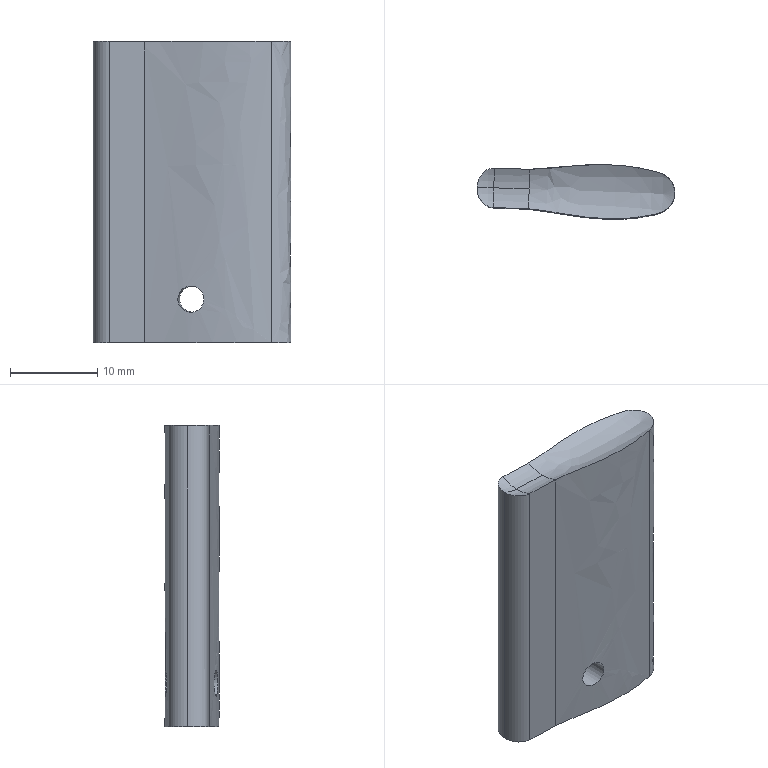Part | NX | features DIE-10 2 | 1 solid | 13 faces | volume 3861 mm3 | spline 9 | plane 3 | cylinder 1 | commonest cylinder face diameters 3 x1
STEP:
#1=CARTESIAN_POINT('',(2369.211,-905.218,828.769));
#2=VERTEX_POINT('',#1);
#3=CARTESIAN_POINT('',(2368.841,-905.228,829.937));
#4=CARTESIAN_POINT('',(2369.375,-905.214,828.774));
#5=CARTESIAN_POINT('',(2368.924,-905.225,827.579));
#6=CARTESIAN_POINT('',(2367.764,-905.286,827.056));
#7=CARTESIAN_POINT('',(2366.574,-905.393,827.498));
#8=CARTESIAN_POINT('',(2366.039,-905.455,828.658));
#9=CARTESIAN_POINT('',(2366.49,-905.402,829.851));
#10=CARTESIAN_POINT('',(2367.646,-905.295,830.376));
#11=CARTESIAN_POINT('',(2368.841,-905.228,829.937));
#12=CARTESIAN_POINT('',(2369.375,-905.214,828.774));
#13=CARTESIAN_POINT('',(2368.924,-905.225,827.579));
#14=B_SPLINE_CURVE_WITH_KNOTS('',3,(#3,#4,#5,#6,#7,#8,#9,#10,#11,#12,#13),.UNSPECIFIED.,.T.,.F.,(1,1,1,1,1,1,1,1,1,1,1,1,1,1,1),(-0.003528,-0.002352,-0.001176,0.,0.001176,0.002352,0.003528,0.004703,0.005879,0.007055,0.008231,0.009407,0.01058,0.01176,0.01293),.UNSPECIFIED.);
#15=EDGE_CURVE('',#2,#2,#14,.F.);
#16=ORIENTED_EDGE('',*,*,#15,.T.);
#17=EDGE_LOOP('',(#16));
#18=FACE_BOUND('',#17,.T.);
#19=CARTESIAN_POINT('',(2362.336,-905.735,858.258));
#20=VERTEX_POINT('',#19);
#21=CARTESIAN_POINT('',(2362.326,-905.735,823.716));
#22=VERTEX_POINT('',#21);
#23=CARTESIAN_POINT('',(2362.326,-905.735,823.716));
#24=CARTESIAN_POINT('',(2362.326,-905.735,835.23));
#25=CARTESIAN_POINT('',(2362.326,-905.735,846.744));
#26=CARTESIAN_POINT('',(2362.326,-905.735,858.258));
#27=B_SPLINE_CURVE_WITH_KNOTS('',3,(#23,#24,#25,#26),.UNSPECIFIED.,.F.,.F.,(4,4),(0.5008,0.5009),.UNSPECIFIED.);
#28=EDGE_CURVE('',#20,#22,#27,.F.);
#29=ORIENTED_EDGE('',*,*,#28,.F.);
#30=CARTESIAN_POINT('',(2376.717,-910.889,858.242));
#31=VERTEX_POINT('',#30);
#32=CARTESIAN_POINT('',(2362.326,-905.733,858.259));
#33=CARTESIAN_POINT('',(2364.117,-905.753,858.273));
#34=CARTESIAN_POINT('',(2366.78,-905.29,858.242));
#35=CARTESIAN_POINT('',(2370.346,-905.165,858.25));
#36=CARTESIAN_POINT('',(2372.574,-905.26,858.245));
#37=CARTESIAN_POINT('',(2374.365,-905.458,858.245));
#38=CARTESIAN_POINT('',(2375.69,-905.739,858.242));
#39=CARTESIAN_POINT('',(2377.015,-906.006,858.242));
#40=CARTESIAN_POINT('',(2378.275,-906.597,858.245));
#41=CARTESIAN_POINT('',(2379.025,-907.857,858.249));
#42=CARTESIAN_POINT('',(2378.948,-909.291,858.252));
#43=CARTESIAN_POINT('',(2378.038,-910.428,858.242));
#44=CARTESIAN_POINT('',(2377.168,-910.778,858.243));
#45=CARTESIAN_POINT('',(2376.717,-910.889,858.242));
#46=B_SPLINE_CURVE_WITH_KNOTS('',3,(#32,#33,#34,#35,#36,#37,#38,#39,#40,#41,#42,#43,#44,#45),.UNSPECIFIED.,.F.,.F.,(4,1,1,1,1,1,1,1,1,1,1,4),(0.,0.005363,0.008044,0.01073,0.01207,0.01341,0.01475,0.01609,0.01743,0.01877,0.02011,0.02145),.UNSPECIFIED.);
#47=EDGE_CURVE('',#20,#31,#46,.T.);
#48=ORIENTED_EDGE('',*,*,#47,.T.);
#49=CARTESIAN_POINT('',(2376.717,-910.889,823.716));
#50=VERTEX_POINT('',#49);
#51=CARTESIAN_POINT('',(2376.717,-910.889,841.133));
#52=DIRECTION('',(0.,0.,-1.));
#53=VECTOR('',#52,1000.);
#54=LINE('',#51,#53);
#55=EDGE_CURVE('',#31,#50,#54,.T.);
#56=ORIENTED_EDGE('',*,*,#55,.T.);
#57=CARTESIAN_POINT('',(2376.717,-910.889,823.716));
#58=CARTESIAN_POINT('',(2377.157,-910.781,823.716));
#59=CARTESIAN_POINT('',(2378.004,-910.446,823.716));
#60=CARTESIAN_POINT('',(2378.916,-909.351,823.716));
#61=CARTESIAN_POINT('',(2379.041,-907.939,823.716));
#62=CARTESIAN_POINT('',(2378.354,-906.687,823.716));
#63=CARTESIAN_POINT('',(2377.143,-906.031,823.716));
#64=CARTESIAN_POINT('',(2375.357,-905.671,823.716));
#65=CARTESIAN_POINT('',(2373.14,-905.263,823.716));
#66=CARTESIAN_POINT('',(2370.412,-905.171,823.716));
#67=CARTESIAN_POINT('',(2366.815,-905.282,823.716));
#68=CARTESIAN_POINT('',(2364.119,-905.753,823.716));
#69=CARTESIAN_POINT('',(2362.326,-905.733,823.716));
#70=B_SPLINE_CURVE_WITH_KNOTS('',3,(#57,#58,#59,#60,#61,#62,#63,#64,#65,#66,#67,#68,#69),.UNSPECIFIED.,.F.,.F.,(4,1,1,1,1,1,1,1,1,1,4),(0.02457,0.02592,0.02728,0.02864,0.03,0.03136,0.03272,0.03544,0.03816,0.04087,0.04631),.UNSPECIFIED.);
#71=EDGE_CURVE('',#50,#22,#70,.T.);
#72=ORIENTED_EDGE('',*,*,#71,.T.);
#73=EDGE_LOOP('',(#29,#48,#56,#72));
#74=FACE_BOUND('',#73,.T.);
#75=CARTESIAN_POINT('',(2362.17,-905.731,858.466));
#76=CARTESIAN_POINT('',(2362.17,-905.731,823.505));
#77=CARTESIAN_POINT('',(2363.26,-905.749,858.475));
#78=CARTESIAN_POINT('',(2363.26,-905.749,823.513));
#79=CARTESIAN_POINT('',(2365.476,-905.528,858.464));
#80=CARTESIAN_POINT('',(2365.476,-905.528,823.503));
#81=CARTESIAN_POINT('',(2368.424,-905.2,858.469));
#82=CARTESIAN_POINT('',(2368.424,-905.2,823.508));
#83=CARTESIAN_POINT('',(2371.439,-905.18,858.468));
#84=CARTESIAN_POINT('',(2371.439,-905.18,823.507));
#85=CARTESIAN_POINT('',(2373.938,-905.364,858.469));
#86=CARTESIAN_POINT('',(2373.938,-905.364,823.508));
#87=CARTESIAN_POINT('',(2375.811,-905.764,858.467));
#88=CARTESIAN_POINT('',(2375.811,-905.764,823.505));
#89=CARTESIAN_POINT('',(2377.335,-906.1,858.467));
#90=CARTESIAN_POINT('',(2377.335,-906.1,823.506));
#91=CARTESIAN_POINT('',(2378.205,-906.616,858.465));
#92=CARTESIAN_POINT('',(2378.205,-906.616,823.504));
#93=CARTESIAN_POINT('',(2378.888,-907.59,858.467));
#94=CARTESIAN_POINT('',(2378.888,-907.59,823.506));
#95=CARTESIAN_POINT('',(2379.023,-908.675,858.467));
#96=CARTESIAN_POINT('',(2379.023,-908.675,823.505));
#97=CARTESIAN_POINT('',(2378.683,-909.662,858.466));
#98=CARTESIAN_POINT('',(2378.683,-909.662,823.504));
#99=CARTESIAN_POINT('',(2377.849,-910.512,858.465));
#100=CARTESIAN_POINT('',(2377.849,-910.512,823.504));
#101=CARTESIAN_POINT('',(2377.168,-910.778,858.467));
#102=CARTESIAN_POINT('',(2377.168,-910.778,823.505));
#103=CARTESIAN_POINT('',(2376.717,-910.889,858.467));
#104=CARTESIAN_POINT('',(2376.717,-910.889,823.506));
#105=B_SPLINE_SURFACE_WITH_KNOTS('',3,1,((#75,#76),(#77,#78),(#79,#80),(#81,#82),(#83,#84),(#85,#86),(#87,#88),(#89,#90),(#91,#92),(#93,#94),(#95,#96),(#97,#98),(#99,#100),(#101,#102),(#103,#104)),.SURF_OF_LINEAR_EXTRUSION.,.F.,.F.,.F.,(4,1,1,1,1,1,1,1,1,1,1,1,4),(2,2),(-0.00628,0.1193,0.2448,0.3704,0.4959,0.5587,0.6215,0.6843,0.747,0.8098,0.8726,0.9354,0.9981),(0.,1.),.UNSPECIFIED.);
#106=ADVANCED_FACE('',(#18,#74),#105,.T.);
#107=CARTESIAN_POINT('',(2369.,-911.248,828.769));
#108=VERTEX_POINT('',#107);
#109=CARTESIAN_POINT('',(2368.714,-911.221,827.578));
#110=CARTESIAN_POINT('',(2369.164,-911.264,828.775));
#111=CARTESIAN_POINT('',(2368.633,-911.213,829.935));
#112=CARTESIAN_POINT('',(2367.447,-911.063,830.376));
#113=CARTESIAN_POINT('',(2366.3,-910.873,829.853));
#114=CARTESIAN_POINT('',(2365.853,-910.788,828.658));
#115=CARTESIAN_POINT('',(2366.38,-910.888,827.5));
#116=CARTESIAN_POINT('',(2367.559,-911.079,827.056));
#117=CARTESIAN_POINT('',(2368.714,-911.221,827.578));
#118=CARTESIAN_POINT('',(2369.164,-911.264,828.775));
#119=CARTESIAN_POINT('',(2368.633,-911.213,829.935));
#120=B_SPLINE_CURVE_WITH_KNOTS('',3,(#109,#110,#111,#112,#113,#114,#115,#116,#117,#118,#119),.UNSPECIFIED.,.T.,.F.,(1,1,1,1,1,1,1,1,1,1,1,1,1,1,1),(-0.003528,-0.002352,-0.001176,0.,0.001176,0.002352,0.003528,0.004704,0.005879,0.007055,0.008231,0.009407,0.01058,0.01176,0.01293),.UNSPECIFIED.);
#121=EDGE_CURVE('',#108,#108,#120,.F.);
#122=ORIENTED_EDGE('',*,*,#121,.T.);
#123=EDGE_LOOP('',(#122));
#124=FACE_BOUND('',#123,.T.);
#125=ORIENTED_EDGE('',*,*,#55,.F.);
#126=CARTESIAN_POINT('',(2362.184,-910.261,858.258));
#127=VERTEX_POINT('',#126);
#128=CARTESIAN_POINT('',(2376.717,-910.889,858.242));
#129=CARTESIAN_POINT('',(2375.519,-911.158,858.226));
#130=CARTESIAN_POINT('',(2373.113,-911.498,858.253));
#131=CARTESIAN_POINT('',(2369.446,-911.36,858.244));
#132=CARTESIAN_POINT('',(2365.815,-910.809,858.245));
#133=CARTESIAN_POINT('',(2363.413,-910.336,858.267));
#134=CARTESIAN_POINT('',(2362.189,-910.262,858.258));
#135=B_SPLINE_CURVE_WITH_KNOTS('',3,(#128,#129,#130,#131,#132,#133,#134),.UNSPECIFIED.,.F.,.F.,(4,1,1,1,4),(0.,0.003638,0.007277,0.01092,0.01455),.UNSPECIFIED.);
#136=EDGE_CURVE('',#31,#127,#135,.T.);
#137=ORIENTED_EDGE('',*,*,#136,.T.);
#138=CARTESIAN_POINT('',(2362.185,-910.261,857.716));
#139=VERTEX_POINT('',#138);
#140=CARTESIAN_POINT('',(2362.179,-910.261,857.716));
#141=CARTESIAN_POINT('',(2362.179,-910.261,857.897));
#142=CARTESIAN_POINT('',(2362.179,-910.261,858.078));
#143=CARTESIAN_POINT('',(2362.179,-910.261,858.258));
#144=B_SPLINE_CURVE_WITH_KNOTS('',3,(#140,#141,#142,#143),.UNSPECIFIED.,.F.,.F.,(4,4),(0.,0.3599),.UNSPECIFIED.);
#145=EDGE_CURVE('',#127,#139,#144,.F.);
#146=ORIENTED_EDGE('',*,*,#145,.T.);
#147=CARTESIAN_POINT('',(2362.196,-910.262,823.716));
#148=VERTEX_POINT('',#147);
#149=CARTESIAN_POINT('',(2362.202,-910.262,823.716));
#150=CARTESIAN_POINT('',(2362.199,-910.261,835.05));
#151=CARTESIAN_POINT('',(2362.195,-910.261,846.383));
#152=CARTESIAN_POINT('',(2362.192,-910.261,857.716));
#153=B_SPLINE_CURVE_WITH_KNOTS('',3,(#149,#150,#151,#152),.UNSPECIFIED.,.F.,.F.,(4,4),(0.,1.),.UNSPECIFIED.);
#154=EDGE_CURVE('',#139,#148,#153,.F.);
#155=ORIENTED_EDGE('',*,*,#154,.T.);
#156=CARTESIAN_POINT('',(2362.196,-910.262,823.716));
#157=CARTESIAN_POINT('',(2363.419,-910.337,823.716));
#158=CARTESIAN_POINT('',(2365.818,-910.807,823.716));
#159=CARTESIAN_POINT('',(2370.65,-911.555,823.716));
#160=CARTESIAN_POINT('',(2374.335,-911.423,823.716));
#161=CARTESIAN_POINT('',(2376.717,-910.889,823.716));
#162=B_SPLINE_CURVE_WITH_KNOTS('',3,(#156,#157,#158,#159,#160,#161),.UNSPECIFIED.,.F.,.F.,(4,1,1,4),(0.02991,0.03359,0.03727,0.04462),.UNSPECIFIED.);
#163=EDGE_CURVE('',#148,#50,#162,.T.);
#164=ORIENTED_EDGE('',*,*,#163,.T.);
#165=EDGE_LOOP('',(#125,#137,#146,#155,#164));
#166=FACE_BOUND('',#165,.T.);
#167=CARTESIAN_POINT('',(2376.717,-910.889,858.483));
#168=CARTESIAN_POINT('',(2376.717,-910.889,823.509));
#169=CARTESIAN_POINT('',(2376.089,-911.03,858.483));
#170=CARTESIAN_POINT('',(2376.089,-911.03,823.509));
#171=CARTESIAN_POINT('',(2374.973,-911.262,858.484));
#172=CARTESIAN_POINT('',(2374.973,-911.262,823.509));
#173=CARTESIAN_POINT('',(2372.578,-911.457,858.484));
#174=CARTESIAN_POINT('',(2372.578,-911.457,823.509));
#175=CARTESIAN_POINT('',(2369.574,-911.374,858.484));
#176=CARTESIAN_POINT('',(2369.574,-911.374,823.509));
#177=CARTESIAN_POINT('',(2365.952,-910.842,858.483));
#178=CARTESIAN_POINT('',(2365.952,-910.842,823.508));
#179=CARTESIAN_POINT('',(2363.495,-910.342,858.483));
#180=CARTESIAN_POINT('',(2363.495,-910.342,823.509));
#181=CARTESIAN_POINT('',(2362.077,-910.255,858.483));
#182=CARTESIAN_POINT('',(2362.077,-910.255,823.509));
#183=B_SPLINE_SURFACE_WITH_KNOTS('',3,1,((#167,#168),(#169,#170),(#171,#172),(#173,#174),(#175,#176),(#177,#178),(#179,#180),(#181,#182)),.SURF_OF_LINEAR_EXTRUSION.,.F.,.F.,.F.,(4,1,1,1,1,4),(2,2),(-0.002152,0.124,0.2502,0.5026,0.755,1.007),(0.,1.),.UNSPECIFIED.);
#184=ADVANCED_FACE('',(#124,#166),#183,.T.);
#185=CARTESIAN_POINT('',(2358.287,-905.594,858.258));
#186=VERTEX_POINT('',#185);
#187=CARTESIAN_POINT('',(2358.286,-905.594,823.716));
#188=VERTEX_POINT('',#187);
#189=CARTESIAN_POINT('',(2358.287,-905.594,858.258));
#190=CARTESIAN_POINT('',(2358.287,-905.594,846.744));
#191=CARTESIAN_POINT('',(2358.287,-905.594,835.23));
#192=CARTESIAN_POINT('',(2358.287,-905.594,823.716));
#193=B_SPLINE_CURVE_WITH_KNOTS('',3,(#189,#190,#191,#192),.UNSPECIFIED.,.F.,.F.,(4,4),(0.4991,0.4992),.UNSPECIFIED.);
#194=EDGE_CURVE('',#186,#188,#193,.T.);
#195=ORIENTED_EDGE('',*,*,#194,.F.);
#196=CARTESIAN_POINT('',(2358.287,-905.594,858.258));
#197=CARTESIAN_POINT('',(2359.636,-905.641,858.258));
#198=CARTESIAN_POINT('',(2360.986,-905.689,858.258));
#199=CARTESIAN_POINT('',(2362.335,-905.736,858.258));
#200=B_SPLINE_CURVE_WITH_KNOTS('',3,(#196,#197,#198,#199),.UNSPECIFIED.,.F.,.F.,(4,4),(0.,0.004051),.UNSPECIFIED.);
#201=EDGE_CURVE('',#186,#20,#200,.T.);
#202=ORIENTED_EDGE('',*,*,#201,.T.);
#203=ORIENTED_EDGE('',*,*,#28,.T.);
#204=CARTESIAN_POINT('',(2362.269,-905.733,823.716));
#205=DIRECTION('',(-0.9994,0.0349,0.));
#206=VECTOR('',#205,1000.);
#207=LINE('',#204,#206);
#208=EDGE_CURVE('',#22,#188,#207,.T.);
#209=ORIENTED_EDGE('',*,*,#208,.T.);
#210=EDGE_LOOP('',(#195,#202,#203,#209));
#211=FACE_BOUND('',#210,.T.);
#212=CARTESIAN_POINT('',(2362.269,-905.733,858.55));
#213=DIRECTION('',(0.0349,0.9994,0.));
#214=DIRECTION('',(-0.9994,0.0349,0.));
#215=AXIS2_PLACEMENT_3D('',#212,#213,#214);
#216=PLANE('',#215);
#217=ADVANCED_FACE('',(#211),#216,.T.);
#218=CARTESIAN_POINT('',(2356.311,-907.791,858.196));
#219=VERTEX_POINT('',#218);
#220=CARTESIAN_POINT('',(2358.286,-905.594,858.258));
#221=CARTESIAN_POINT('',(2357.734,-905.574,858.259));
#222=CARTESIAN_POINT('',(2356.678,-906.139,858.228));
#223=CARTESIAN_POINT('',(2356.332,-907.24,858.195));
#224=CARTESIAN_POINT('',(2356.311,-907.79,858.196));
#225=B_SPLINE_CURVE_WITH_KNOTS('',3,(#220,#221,#222,#223,#224),.UNSPECIFIED.,.F.,.F.,(4,1,4),(0.,0.001633,0.003266),.UNSPECIFIED.);
#226=EDGE_CURVE('',#186,#219,#225,.T.);
#227=ORIENTED_EDGE('',*,*,#226,.F.);
#228=ORIENTED_EDGE('',*,*,#194,.T.);
#229=CARTESIAN_POINT('',(2356.311,-907.79,823.716));
#230=VERTEX_POINT('',#229);
#231=CARTESIAN_POINT('',(2358.286,-905.594,823.716));
#232=CARTESIAN_POINT('',(2357.734,-905.574,823.716));
#233=CARTESIAN_POINT('',(2356.678,-906.138,823.716));
#234=CARTESIAN_POINT('',(2356.332,-907.241,823.716));
#235=CARTESIAN_POINT('',(2356.311,-907.79,823.716));
#236=B_SPLINE_CURVE_WITH_KNOTS('',3,(#231,#232,#233,#234,#235),.UNSPECIFIED.,.F.,.F.,(4,1,4),(0.03107,0.03273,0.03439),.UNSPECIFIED.);
#237=EDGE_CURVE('',#188,#230,#236,.T.);
#238=ORIENTED_EDGE('',*,*,#237,.T.);
#239=CARTESIAN_POINT('',(2356.311,-907.793,858.196));
#240=CARTESIAN_POINT('',(2356.311,-907.793,846.703));
#241=CARTESIAN_POINT('',(2356.311,-907.793,835.21));
#242=CARTESIAN_POINT('',(2356.311,-907.793,823.716));
#243=B_SPLINE_CURVE_WITH_KNOTS('',3,(#239,#240,#241,#242),.UNSPECIFIED.,.F.,.F.,(4,4),(0.4991,0.4992),.UNSPECIFIED.);
#244=EDGE_CURVE('',#219,#230,#243,.T.);
#245=ORIENTED_EDGE('',*,*,#244,.F.);
#246=EDGE_LOOP('',(#227,#228,#238,#245));
#247=FACE_BOUND('',#246,.T.);
#248=CARTESIAN_POINT('',(2356.311,-907.793,858.432));
#249=CARTESIAN_POINT('',(2356.311,-907.793,823.476));
#250=CARTESIAN_POINT('',(2356.318,-907.615,858.432));
#251=CARTESIAN_POINT('',(2356.318,-907.615,823.476));
#252=CARTESIAN_POINT('',(2356.349,-907.359,858.433));
#253=CARTESIAN_POINT('',(2356.349,-907.359,823.477));
#254=CARTESIAN_POINT('',(2356.509,-906.778,858.439));
#255=CARTESIAN_POINT('',(2356.509,-906.778,823.482));
#256=CARTESIAN_POINT('',(2356.874,-906.172,858.451));
#257=CARTESIAN_POINT('',(2356.874,-906.172,823.494));
#258=CARTESIAN_POINT('',(2357.409,-905.766,858.46));
#259=CARTESIAN_POINT('',(2357.409,-905.766,823.504));
#260=CARTESIAN_POINT('',(2357.922,-905.61,858.465));
#261=CARTESIAN_POINT('',(2357.922,-905.61,823.508));
#262=CARTESIAN_POINT('',(2358.126,-905.588,858.466));
#263=CARTESIAN_POINT('',(2358.126,-905.588,823.509));
#264=CARTESIAN_POINT('',(2358.286,-905.594,858.465));
#265=CARTESIAN_POINT('',(2358.286,-905.594,823.509));
#266=B_SPLINE_SURFACE_WITH_KNOTS('',3,1,((#248,#249),(#250,#251),(#252,#253),(#254,#255),(#256,#257),(#258,#259),(#260,#261),(#262,#263),(#264,#265)),.SURF_OF_LINEAR_EXTRUSION.,.F.,.F.,.F.,(4,1,1,1,1,1,4),(2,2),(0.0001248,0.1252,0.2502,0.5002,0.7503,0.8753,1.),(0.,1.),.UNSPECIFIED.);
#267=ADVANCED_FACE('',(#247),#266,.T.);
#268=CARTESIAN_POINT('',(2358.132,-910.119,858.258));
#269=VERTEX_POINT('',#268);
#270=CARTESIAN_POINT('',(2358.134,-910.119,823.716));
#271=VERTEX_POINT('',#270);
#272=CARTESIAN_POINT('',(2358.134,-910.119,823.716));
#273=CARTESIAN_POINT('',(2358.134,-910.119,835.23));
#274=CARTESIAN_POINT('',(2358.134,-910.119,846.744));
#275=CARTESIAN_POINT('',(2358.134,-910.119,858.258));
#276=B_SPLINE_CURVE_WITH_KNOTS('',3,(#272,#273,#274,#275),.UNSPECIFIED.,.F.,.F.,(4,4),(0.5008,0.5009),.UNSPECIFIED.);
#277=EDGE_CURVE('',#269,#271,#276,.F.);
#278=ORIENTED_EDGE('',*,*,#277,.F.);
#279=CARTESIAN_POINT('',(2358.135,-910.119,858.258));
#280=CARTESIAN_POINT('',(2357.581,-910.099,858.258));
#281=CARTESIAN_POINT('',(2356.564,-909.466,858.228));
#282=CARTESIAN_POINT('',(2356.292,-908.341,858.196));
#283=CARTESIAN_POINT('',(2356.311,-907.79,858.196));
#284=B_SPLINE_CURVE_WITH_KNOTS('',3,(#279,#280,#281,#282,#283),.UNSPECIFIED.,.F.,.F.,(4,1,4),(0.,0.001637,0.003275),.UNSPECIFIED.);
#285=EDGE_CURVE('',#269,#219,#284,.T.);
#286=ORIENTED_EDGE('',*,*,#285,.T.);
#287=ORIENTED_EDGE('',*,*,#244,.T.);
#288=CARTESIAN_POINT('',(2358.134,-910.119,823.716));
#289=CARTESIAN_POINT('',(2357.581,-910.099,823.716));
#290=CARTESIAN_POINT('',(2356.565,-909.468,823.716));
#291=CARTESIAN_POINT('',(2356.292,-908.34,823.716));
#292=CARTESIAN_POINT('',(2356.311,-907.79,823.716));
#293=B_SPLINE_CURVE_WITH_KNOTS('',3,(#288,#289,#290,#291,#292),.UNSPECIFIED.,.F.,.F.,(4,1,4),(0.05975,0.06141,0.06307),.UNSPECIFIED.);
#294=EDGE_CURVE('',#271,#230,#293,.T.);
#295=ORIENTED_EDGE('',*,*,#294,.F.);
#296=EDGE_LOOP('',(#278,#286,#287,#295));
#297=FACE_BOUND('',#296,.T.);
#298=CARTESIAN_POINT('',(2358.135,-910.119,858.465));
#299=CARTESIAN_POINT('',(2358.135,-910.119,823.509));
#300=CARTESIAN_POINT('',(2358.035,-910.115,858.465));
#301=CARTESIAN_POINT('',(2358.035,-910.115,823.509));
#302=CARTESIAN_POINT('',(2357.955,-910.106,858.465));
#303=CARTESIAN_POINT('',(2357.955,-910.106,823.509));
#304=CARTESIAN_POINT('',(2357.678,-910.051,858.464));
#305=CARTESIAN_POINT('',(2357.678,-910.051,823.508));
#306=CARTESIAN_POINT('',(2357.279,-909.886,858.461));
#307=CARTESIAN_POINT('',(2357.279,-909.886,823.504));
#308=CARTESIAN_POINT('',(2356.755,-909.445,858.451));
#309=CARTESIAN_POINT('',(2356.755,-909.445,823.494));
#310=CARTESIAN_POINT('',(2356.375,-908.681,858.437));
#311=CARTESIAN_POINT('',(2356.375,-908.681,823.48));
#312=CARTESIAN_POINT('',(2356.3,-908.088,858.432));
#313=CARTESIAN_POINT('',(2356.3,-908.088,823.476));
#314=CARTESIAN_POINT('',(2356.311,-907.79,858.432));
#315=CARTESIAN_POINT('',(2356.311,-907.79,823.476));
#316=B_SPLINE_SURFACE_WITH_KNOTS('',3,1,((#298,#299),(#300,#301),(#302,#303),(#304,#305),(#306,#307),(#308,#309),(#310,#311),(#312,#313),(#314,#315)),.SURF_OF_LINEAR_EXTRUSION.,.F.,.F.,.F.,(4,1,1,1,1,1,4),(2,2),(0.0008005,0.06324,0.1257,0.2506,0.5003,0.7501,0.9999),(0.,1.),.UNSPECIFIED.);
#317=ADVANCED_FACE('',(#297),#316,.T.);
#318=CARTESIAN_POINT('',(2362.189,-910.261,858.258));
#319=CARTESIAN_POINT('',(2360.838,-910.214,858.258));
#320=CARTESIAN_POINT('',(2359.486,-910.167,858.258));
#321=CARTESIAN_POINT('',(2358.134,-910.119,858.258));
#322=B_SPLINE_CURVE_WITH_KNOTS('',3,(#318,#319,#320,#321),.UNSPECIFIED.,.F.,.F.,(4,4),(0.,0.004058),.UNSPECIFIED.);
#323=EDGE_CURVE('',#127,#269,#322,.T.);
#324=ORIENTED_EDGE('',*,*,#323,.F.);
#325=CARTESIAN_POINT('',(2362.273,-907.996,857.716));
#326=VERTEX_POINT('',#325);
#327=CARTESIAN_POINT('',(2362.189,-910.261,858.258));
#328=CARTESIAN_POINT('',(2362.216,-909.488,857.866));
#329=CARTESIAN_POINT('',(2362.244,-908.699,857.716));
#330=CARTESIAN_POINT('',(2362.268,-907.999,857.716));
#331=B_SPLINE_CURVE_WITH_KNOTS('',3,(#327,#328,#329,#330),.UNSPECIFIED.,.F.,.F.,(4,4),(0.1786,1.),.UNSPECIFIED.);
#332=EDGE_CURVE('',#127,#326,#331,.T.);
#333=ORIENTED_EDGE('',*,*,#332,.T.);
#334=CARTESIAN_POINT('',(2358.21,-907.856,857.716));
#335=VERTEX_POINT('',#334);
#336=CARTESIAN_POINT('',(2362.268,-907.999,857.716));
#337=CARTESIAN_POINT('',(2360.915,-907.951,857.716));
#338=CARTESIAN_POINT('',(2359.562,-907.904,857.716));
#339=CARTESIAN_POINT('',(2358.21,-907.857,857.716));
#340=B_SPLINE_CURVE_WITH_KNOTS('',3,(#336,#337,#338,#339),.UNSPECIFIED.,.F.,.F.,(4,4),(0.,0.9999),.UNSPECIFIED.);
#341=EDGE_CURVE('',#335,#326,#340,.F.);
#342=ORIENTED_EDGE('',*,*,#341,.F.);
#343=CARTESIAN_POINT('',(2358.209,-907.857,857.716));
#344=CARTESIAN_POINT('',(2358.185,-908.557,857.716));
#345=CARTESIAN_POINT('',(2358.157,-909.347,857.866));
#346=CARTESIAN_POINT('',(2358.13,-910.119,858.258));
#347=B_SPLINE_CURVE_WITH_KNOTS('',3,(#343,#344,#345,#346),.UNSPECIFIED.,.F.,.F.,(4,4),(0.,0.8214),.UNSPECIFIED.);
#348=EDGE_CURVE('',#269,#335,#347,.F.);
#349=ORIENTED_EDGE('',*,*,#348,.F.);
#350=EDGE_LOOP('',(#324,#333,#342,#349));
#351=FACE_BOUND('',#350,.T.);
#352=CARTESIAN_POINT('',(2358.209,-907.857,857.716));
#353=CARTESIAN_POINT('',(2358.185,-908.561,857.716));
#354=CARTESIAN_POINT('',(2358.157,-909.355,857.867));
#355=CARTESIAN_POINT('',(2358.13,-910.133,858.265));
#356=CARTESIAN_POINT('',(2359.562,-907.904,857.716));
#357=CARTESIAN_POINT('',(2359.538,-908.609,857.716));
#358=CARTESIAN_POINT('',(2359.51,-909.403,857.867));
#359=CARTESIAN_POINT('',(2359.483,-910.18,858.265));
#360=CARTESIAN_POINT('',(2360.915,-907.951,857.716));
#361=CARTESIAN_POINT('',(2360.891,-908.656,857.716));
#362=CARTESIAN_POINT('',(2360.863,-909.45,857.867));
#363=CARTESIAN_POINT('',(2360.836,-910.228,858.265));
#364=CARTESIAN_POINT('',(2362.268,-907.999,857.716));
#365=CARTESIAN_POINT('',(2362.244,-908.703,857.716));
#366=CARTESIAN_POINT('',(2362.216,-909.497,857.867));
#367=CARTESIAN_POINT('',(2362.189,-910.275,858.265));
#368=B_SPLINE_SURFACE_WITH_KNOTS('',3,3,((#352,#353,#354,#355),(#356,#357,#358,#359),(#360,#361,#362,#363),(#364,#365,#366,#367)),.UNSPECIFIED.,.F.,.F.,.F.,(4,4),(4,4),(0.,1.),(0.,0.8263),.UNSPECIFIED.);
#369=ADVANCED_FACE('',(#351),#368,.F.);
#370=ORIENTED_EDGE('',*,*,#47,.F.);
#371=CARTESIAN_POINT('',(2362.347,-905.736,858.258));
#372=CARTESIAN_POINT('',(2362.324,-906.365,857.939));
#373=CARTESIAN_POINT('',(2362.298,-907.139,857.717));
#374=CARTESIAN_POINT('',(2362.268,-907.995,857.716));
#375=B_SPLINE_CURVE_WITH_KNOTS('',3,(#371,#372,#373,#374),.UNSPECIFIED.,.F.,.F.,(4,4),(0.1357,1.),.UNSPECIFIED.);
#376=EDGE_CURVE('',#326,#20,#375,.F.);
#377=ORIENTED_EDGE('',*,*,#376,.F.);
#378=ORIENTED_EDGE('',*,*,#332,.F.);
#379=ORIENTED_EDGE('',*,*,#136,.F.);
#380=EDGE_LOOP('',(#370,#377,#378,#379));
#381=FACE_BOUND('',#380,.T.);
#382=CARTESIAN_POINT('',(2362.217,-905.015,858.702));
#383=CARTESIAN_POINT('',(2362.967,-905.006,858.724));
#384=CARTESIAN_POINT('',(2364.154,-905.023,858.66));
#385=CARTESIAN_POINT('',(2366.181,-905.092,858.438));
#386=CARTESIAN_POINT('',(2368.134,-905.122,858.319));
#387=CARTESIAN_POINT('',(2370.186,-905.138,858.272));
#388=CARTESIAN_POINT('',(2372.137,-905.135,858.3));
#389=CARTESIAN_POINT('',(2373.81,-905.115,858.401));
#390=CARTESIAN_POINT('',(2375.054,-905.116,858.525));
#391=CARTESIAN_POINT('',(2375.896,-905.11,858.654));
#392=CARTESIAN_POINT('',(2376.466,-905.105,858.755));
#393=CARTESIAN_POINT('',(2376.951,-905.089,858.848));
#394=CARTESIAN_POINT('',(2377.784,-905.091,859.009));
#395=CARTESIAN_POINT('',(2378.57,-905.189,859.24));
#396=CARTESIAN_POINT('',(2379.025,-905.272,859.465));
#397=CARTESIAN_POINT('',(2362.232,-905.447,858.38));
#398=CARTESIAN_POINT('',(2362.966,-905.43,858.408));
#399=CARTESIAN_POINT('',(2364.169,-905.459,858.349));
#400=CARTESIAN_POINT('',(2366.18,-905.547,858.159));
#401=CARTESIAN_POINT('',(2368.127,-905.59,858.05));
#402=CARTESIAN_POINT('',(2370.173,-905.613,858.004));
#403=CARTESIAN_POINT('',(2372.12,-905.62,858.02));
#404=CARTESIAN_POINT('',(2373.779,-905.608,858.096));
#405=CARTESIAN_POINT('',(2375.026,-905.602,858.211));
#406=CARTESIAN_POINT('',(2375.854,-905.594,858.321));
#407=CARTESIAN_POINT('',(2376.441,-905.578,858.422));
#408=CARTESIAN_POINT('',(2376.903,-905.554,858.504));
#409=CARTESIAN_POINT('',(2377.791,-905.555,858.653));
#410=CARTESIAN_POINT('',(2378.599,-905.659,858.898));
#411=CARTESIAN_POINT('',(2379.061,-905.753,859.13));
#412=CARTESIAN_POINT('',(2362.223,-906.185,858.001));
#413=CARTESIAN_POINT('',(2362.953,-906.168,858.019));
#414=CARTESIAN_POINT('',(2364.182,-906.2,857.971));
#415=CARTESIAN_POINT('',(2366.17,-906.283,857.826));
#416=CARTESIAN_POINT('',(2368.108,-906.336,857.73));
#417=CARTESIAN_POINT('',(2370.151,-906.367,857.683));
#418=CARTESIAN_POINT('',(2372.086,-906.391,857.683));
#419=CARTESIAN_POINT('',(2373.739,-906.394,857.732));
#420=CARTESIAN_POINT('',(2374.952,-906.377,857.81));
#421=CARTESIAN_POINT('',(2375.774,-906.337,857.898));
#422=CARTESIAN_POINT('',(2376.34,-906.293,857.972));
#423=CARTESIAN_POINT('',(2376.905,-906.287,858.038));
#424=CARTESIAN_POINT('',(2377.804,-906.348,858.156));
#425=CARTESIAN_POINT('',(2378.692,-906.463,858.459));
#426=CARTESIAN_POINT('',(2379.126,-906.514,858.726));
#427=CARTESIAN_POINT('',(2362.203,-907.219,857.756));
#428=CARTESIAN_POINT('',(2362.942,-907.22,857.764));
#429=CARTESIAN_POINT('',(2364.16,-907.261,857.72));
#430=CARTESIAN_POINT('',(2366.145,-907.329,857.598));
#431=CARTESIAN_POINT('',(2368.075,-907.388,857.509));
#432=CARTESIAN_POINT('',(2370.115,-907.432,857.458));
#433=CARTESIAN_POINT('',(2372.049,-907.48,857.447));
#434=CARTESIAN_POINT('',(2373.68,-907.521,857.474));
#435=CARTESIAN_POINT('',(2374.867,-907.524,857.511));
#436=CARTESIAN_POINT('',(2375.67,-907.511,857.546));
#437=CARTESIAN_POINT('',(2376.283,-907.509,857.583));
#438=CARTESIAN_POINT('',(2376.894,-907.527,857.639));
#439=CARTESIAN_POINT('',(2377.847,-907.574,857.803));
#440=CARTESIAN_POINT('',(2378.641,-907.609,858.109));
#441=CARTESIAN_POINT('',(2379.115,-907.649,858.38));
#442=CARTESIAN_POINT('',(2362.177,-908.003,857.696));
#443=CARTESIAN_POINT('',(2362.921,-908.028,857.699));
#444=CARTESIAN_POINT('',(2364.137,-908.07,857.659));
#445=CARTESIAN_POINT('',(2366.119,-908.13,857.541));
#446=CARTESIAN_POINT('',(2368.048,-908.193,857.452));
#447=CARTESIAN_POINT('',(2370.087,-908.249,857.397));
#448=CARTESIAN_POINT('',(2372.021,-908.316,857.385));
#449=CARTESIAN_POINT('',(2373.648,-908.387,857.409));
#450=CARTESIAN_POINT('',(2374.822,-908.432,857.432));
#451=CARTESIAN_POINT('',(2375.628,-908.463,857.454));
#452=CARTESIAN_POINT('',(2376.251,-908.492,857.485));
#453=CARTESIAN_POINT('',(2376.878,-908.521,857.545));
#454=CARTESIAN_POINT('',(2377.814,-908.565,857.712));
#455=CARTESIAN_POINT('',(2378.61,-908.584,858.004));
#456=CARTESIAN_POINT('',(2379.107,-908.587,858.297));
#457=CARTESIAN_POINT('',(2362.149,-908.783,857.758));
#458=CARTESIAN_POINT('',(2362.889,-908.834,857.765));
#459=CARTESIAN_POINT('',(2364.106,-908.88,857.724));
#460=CARTESIAN_POINT('',(2366.089,-908.931,857.599));
#461=CARTESIAN_POINT('',(2368.02,-908.999,857.507));
#462=CARTESIAN_POINT('',(2370.057,-909.068,857.45));
#463=CARTESIAN_POINT('',(2371.997,-909.154,857.441));
#464=CARTESIAN_POINT('',(2373.627,-909.254,857.475));
#465=CARTESIAN_POINT('',(2374.809,-909.338,857.516));
#466=CARTESIAN_POINT('',(2375.619,-909.414,857.559));
#467=CARTESIAN_POINT('',(2376.237,-909.467,857.604));
#468=CARTESIAN_POINT('',(2376.849,-909.508,857.672));
#469=CARTESIAN_POINT('',(2377.786,-909.544,857.847));
#470=CARTESIAN_POINT('',(2378.561,-909.573,858.145));
#471=CARTESIAN_POINT('',(2379.037,-909.572,858.414));
#472=CARTESIAN_POINT('',(2362.098,-909.807,858.004));
#473=CARTESIAN_POINT('',(2362.829,-909.886,858.023));
#474=CARTESIAN_POINT('',(2364.06,-909.942,857.982));
#475=CARTESIAN_POINT('',(2366.041,-909.976,857.828));
#476=CARTESIAN_POINT('',(2367.981,-910.056,857.728));
#477=CARTESIAN_POINT('',(2370.019,-910.145,857.67));
#478=CARTESIAN_POINT('',(2371.963,-910.252,857.671));
#479=CARTESIAN_POINT('',(2373.62,-910.387,857.741));
#480=CARTESIAN_POINT('',(2374.814,-910.487,857.82));
#481=CARTESIAN_POINT('',(2375.659,-910.57,857.915));
#482=CARTESIAN_POINT('',(2376.236,-910.654,858.004));
#483=CARTESIAN_POINT('',(2376.803,-910.705,858.09));
#484=CARTESIAN_POINT('',(2377.7,-910.728,858.248));
#485=CARTESIAN_POINT('',(2378.527,-910.691,858.545));
#486=CARTESIAN_POINT('',(2378.969,-910.656,858.798));
#487=CARTESIAN_POINT('',(2362.05,-910.54,858.379));
#488=CARTESIAN_POINT('',(2362.803,-910.63,858.418));
#489=CARTESIAN_POINT('',(2363.992,-910.67,858.361));
#490=CARTESIAN_POINT('',(2366.,-910.714,858.163));
#491=CARTESIAN_POINT('',(2367.948,-910.805,858.05));
#492=CARTESIAN_POINT('',(2369.991,-910.912,857.995));
#493=CARTESIAN_POINT('',(2371.939,-911.036,858.011));
#494=CARTESIAN_POINT('',(2373.62,-911.166,858.106));
#495=CARTESIAN_POINT('',(2374.829,-911.269,858.227));
#496=CARTESIAN_POINT('',(2375.679,-911.322,858.336));
#497=CARTESIAN_POINT('',(2376.3,-911.37,858.451));
#498=CARTESIAN_POINT('',(2376.767,-911.427,858.552));
#499=CARTESIAN_POINT('',(2377.65,-911.478,858.735));
#500=CARTESIAN_POINT('',(2378.4,-911.444,858.989));
#501=CARTESIAN_POINT('',(2378.86,-911.398,859.216));
#502=CARTESIAN_POINT('',(2362.015,-910.978,858.708));
#503=CARTESIAN_POINT('',(2362.774,-911.057,858.746));
#504=CARTESIAN_POINT('',(2363.943,-911.104,858.673));
#505=CARTESIAN_POINT('',(2365.971,-911.17,858.443));
#506=CARTESIAN_POINT('',(2367.924,-911.274,858.321));
#507=CARTESIAN_POINT('',(2369.973,-911.397,858.27));
#508=CARTESIAN_POINT('',(2371.924,-911.529,858.296));
#509=CARTESIAN_POINT('',(2373.612,-911.658,858.409));
#510=CARTESIAN_POINT('',(2374.833,-911.752,858.546));
#511=CARTESIAN_POINT('',(2375.677,-911.808,858.67));
#512=CARTESIAN_POINT('',(2376.291,-911.84,858.781));
#513=CARTESIAN_POINT('',(2376.789,-911.888,858.893));
#514=CARTESIAN_POINT('',(2377.615,-911.939,859.089));
#515=CARTESIAN_POINT('',(2378.353,-911.904,859.333));
#516=CARTESIAN_POINT('',(2378.802,-911.865,859.556));
#517=B_SPLINE_SURFACE_WITH_KNOTS('',3,3,((#382,#383,#384,#385,#386,#387,#388,#389,#390,#391,#392,#393,#394,#395,#396),(#397,#398,#399,#400,#401,#402,#403,#404,#405,#406,#407,#408,#409,#410,#411),(#412,#413,#414,#415,#416,#417,#418,#419,#420,#421,#422,#423,#424,#425,#426),(#427,#428,#429,#430,#431,#432,#433,#434,#435,#436,#437,#438,#439,#440,#441),(#442,#443,#444,#445,#446,#447,#448,#449,#450,#451,#452,#453,#454,#455,#456),(#457,#458,#459,#460,#461,#462,#463,#464,#465,#466,#467,#468,#469,#470,#471),(#472,#473,#474,#475,#476,#477,#478,#479,#480,#481,#482,#483,#484,#485,#486),(#487,#488,#489,#490,#491,#492,#493,#494,#495,#496,#497,#498,#499,#500,#501),(#502,#503,#504,#505,#506,#507,#508,#509,#510,#511,#512,#513,#514,#515,#516)),.UNSPECIFIED.,.F.,.F.,.F.,(4,1,1,1,1,1,4),(4,1,1,1,1,1,1,1,1,1,1,1,4),(-0.002149,-0.001071,-0.0005322,0.000006828,0.0005459,0.001085,0.002163),(-0.00784,-0.005513,-0.003851,-0.001856,0.000138,0.002132,0.003794,0.004958,0.005623,0.006121,0.00662,0.007118,0.008116),.UNSPECIFIED.);
#518=ADVANCED_FACE('',(#381),#517,.T.);
#519=ORIENTED_EDGE('',*,*,#201,.F.);
#520=CARTESIAN_POINT('',(2358.288,-905.594,858.258));
#521=CARTESIAN_POINT('',(2358.261,-906.366,857.866));
#522=CARTESIAN_POINT('',(2358.234,-907.156,857.716));
#523=CARTESIAN_POINT('',(2358.209,-907.856,857.716));
#524=B_SPLINE_CURVE_WITH_KNOTS('',3,(#520,#521,#522,#523),.UNSPECIFIED.,.F.,.F.,(4,4),(0.1785,0.9998),.UNSPECIFIED.);
#525=EDGE_CURVE('',#335,#186,#524,.F.);
#526=ORIENTED_EDGE('',*,*,#525,.F.);
#527=ORIENTED_EDGE('',*,*,#341,.T.);
#528=ORIENTED_EDGE('',*,*,#376,.T.);
#529=EDGE_LOOP('',(#519,#526,#527,#528));
#530=FACE_BOUND('',#529,.T.);
#531=CARTESIAN_POINT('',(2358.263,-905.579,858.265));
#532=CARTESIAN_POINT('',(2358.236,-906.357,857.867));
#533=CARTESIAN_POINT('',(2358.208,-907.151,857.716));
#534=CARTESIAN_POINT('',(2358.184,-907.856,857.716));
#535=CARTESIAN_POINT('',(2359.625,-905.627,858.265));
#536=CARTESIAN_POINT('',(2359.597,-906.405,857.867));
#537=CARTESIAN_POINT('',(2359.57,-907.199,857.716));
#538=CARTESIAN_POINT('',(2359.545,-907.903,857.716));
#539=CARTESIAN_POINT('',(2360.986,-905.674,858.265));
#540=CARTESIAN_POINT('',(2360.959,-906.452,857.867));
#541=CARTESIAN_POINT('',(2360.931,-907.246,857.716));
#542=CARTESIAN_POINT('',(2360.907,-907.951,857.716));
#543=CARTESIAN_POINT('',(2362.348,-905.722,858.265));
#544=CARTESIAN_POINT('',(2362.321,-906.5,857.867));
#545=CARTESIAN_POINT('',(2362.293,-907.294,857.716));
#546=CARTESIAN_POINT('',(2362.268,-907.999,857.716));
#547=B_SPLINE_SURFACE_WITH_KNOTS('',3,3,((#531,#532,#533,#534),(#535,#536,#537,#538),(#539,#540,#541,#542),(#543,#544,#545,#546)),.UNSPECIFIED.,.F.,.F.,.F.,(4,4),(4,4),(-0.006325,1.),(0.1736,1.),.UNSPECIFIED.);
#548=ADVANCED_FACE('',(#530),#547,.F.);
#549=ORIENTED_EDGE('',*,*,#525,.T.);
#550=ORIENTED_EDGE('',*,*,#226,.T.);
#551=CARTESIAN_POINT('',(2356.311,-907.79,858.196));
#552=CARTESIAN_POINT('',(2356.891,-907.81,857.883));
#553=CARTESIAN_POINT('',(2357.55,-907.833,857.716));
#554=CARTESIAN_POINT('',(2358.21,-907.856,857.716));
#555=B_SPLINE_CURVE_WITH_KNOTS('',3,(#551,#552,#553,#554),.UNSPECIFIED.,.F.,.F.,(4,4),(0.2504,1.),.UNSPECIFIED.);
#556=EDGE_CURVE('',#335,#219,#555,.F.);
#557=ORIENTED_EDGE('',*,*,#556,.F.);
#558=EDGE_LOOP('',(#549,#550,#557));
#559=FACE_BOUND('',#558,.T.);
#560=CARTESIAN_POINT('',(2356.372,-905.734,858.698));
#561=CARTESIAN_POINT('',(2356.963,-905.609,858.413));
#562=CARTESIAN_POINT('',(2357.633,-905.556,858.263));
#563=CARTESIAN_POINT('',(2358.301,-905.58,858.265));
#564=CARTESIAN_POINT('',(2356.347,-906.455,858.351));
#565=CARTESIAN_POINT('',(2356.936,-906.381,858.042));
#566=CARTESIAN_POINT('',(2357.605,-906.355,857.879));
#567=CARTESIAN_POINT('',(2358.273,-906.379,857.882));
#568=CARTESIAN_POINT('',(2356.323,-907.143,858.186));
#569=CARTESIAN_POINT('',(2356.911,-907.118,857.865));
#570=CARTESIAN_POINT('',(2357.579,-907.117,857.696));
#571=CARTESIAN_POINT('',(2358.246,-907.14,857.699));
#572=CARTESIAN_POINT('',(2356.3,-907.797,858.202));
#573=CARTESIAN_POINT('',(2356.886,-907.818,857.882));
#574=CARTESIAN_POINT('',(2357.554,-907.841,857.714));
#575=CARTESIAN_POINT('',(2358.221,-907.864,857.716));
#576=B_SPLINE_SURFACE_WITH_KNOTS('',3,3,((#560,#561,#562,#563),(#564,#565,#566,#567),(#568,#569,#570,#571),(#572,#573,#574,#575)),.UNSPECIFIED.,.F.,.F.,.F.,(4,4),(4,4),(0.1784,1.005),(0.2458,1.005),.UNSPECIFIED.);
#577=ADVANCED_FACE('',(#559),#576,.T.);
#578=ORIENTED_EDGE('',*,*,#285,.F.);
#579=ORIENTED_EDGE('',*,*,#348,.T.);
#580=ORIENTED_EDGE('',*,*,#556,.T.);
#581=EDGE_LOOP('',(#578,#579,#580));
#582=FACE_BOUND('',#581,.T.);
#583=CARTESIAN_POINT('',(2356.228,-909.845,858.698));
#584=CARTESIAN_POINT('',(2356.808,-910.012,858.411));
#585=CARTESIAN_POINT('',(2357.493,-910.113,858.261));
#586=CARTESIAN_POINT('',(2358.14,-910.133,858.265));
#587=CARTESIAN_POINT('',(2356.253,-909.13,858.353));
#588=CARTESIAN_POINT('',(2356.835,-909.246,858.042));
#589=CARTESIAN_POINT('',(2357.52,-909.32,857.879));
#590=CARTESIAN_POINT('',(2358.168,-909.341,857.884));
#591=CARTESIAN_POINT('',(2356.277,-908.445,858.188));
#592=CARTESIAN_POINT('',(2356.861,-908.512,857.865));
#593=CARTESIAN_POINT('',(2357.547,-908.56,857.696));
#594=CARTESIAN_POINT('',(2358.194,-908.582,857.701));
#595=CARTESIAN_POINT('',(2356.3,-907.79,858.202));
#596=CARTESIAN_POINT('',(2356.885,-907.81,857.88));
#597=CARTESIAN_POINT('',(2357.572,-907.834,857.712));
#598=CARTESIAN_POINT('',(2358.22,-907.857,857.716));
#599=B_SPLINE_SURFACE_WITH_KNOTS('',3,3,((#583,#584,#585,#586),(#587,#588,#589,#590),(#591,#592,#593,#594),(#595,#596,#597,#598)),.UNSPECIFIED.,.F.,.F.,.F.,(4,4),(4,4),(0.1753,1.),(0.2389,1.009),.UNSPECIFIED.);
#600=ADVANCED_FACE('',(#582),#599,.F.);
#601=ORIENTED_EDGE('',*,*,#145,.F.);
#602=ORIENTED_EDGE('',*,*,#323,.T.);
#603=ORIENTED_EDGE('',*,*,#277,.T.);
#604=CARTESIAN_POINT('',(2362.189,-910.261,823.716));
#605=DIRECTION('',(0.9994,-0.0349,0.));
#606=VECTOR('',#605,1000.);
#607=LINE('',#604,#606);
#608=EDGE_CURVE('',#271,#148,#607,.T.);
#609=ORIENTED_EDGE('',*,*,#608,.T.);
#610=ORIENTED_EDGE('',*,*,#154,.F.);
#611=EDGE_LOOP('',(#601,#602,#603,#609,#610));
#612=FACE_BOUND('',#611,.T.);
#613=CARTESIAN_POINT('',(2362.189,-910.261,858.55));
#614=DIRECTION('',(-0.0349,-0.9994,0.));
#615=DIRECTION('',(0.9994,-0.0349,0.));
#616=AXIS2_PLACEMENT_3D('',#613,#614,#615);
#617=PLANE('',#616);
#618=ADVANCED_FACE('',(#612),#617,.T.);
#619=ORIENTED_EDGE('',*,*,#71,.F.);
#620=ORIENTED_EDGE('',*,*,#163,.F.);
#621=ORIENTED_EDGE('',*,*,#608,.F.);
#622=ORIENTED_EDGE('',*,*,#294,.T.);
#623=ORIENTED_EDGE('',*,*,#237,.F.);
#624=ORIENTED_EDGE('',*,*,#208,.F.);
#625=EDGE_LOOP('',(#619,#620,#621,#622,#623,#624));
#626=FACE_BOUND('',#625,.T.);
#627=CARTESIAN_POINT('',(2350.561,-907.752,823.716));
#628=DIRECTION('',(0.,0.,-1.));
#629=DIRECTION('',(-1.,0.,0.));
#630=AXIS2_PLACEMENT_3D('',#627,#628,#629);
#631=PLANE('',#630);
#632=ADVANCED_FACE('',(#626),#631,.T.);
#633=ORIENTED_EDGE('',*,*,#15,.F.);
#634=EDGE_LOOP('',(#633));
#635=FACE_BOUND('',#634,.T.);
#636=ORIENTED_EDGE('',*,*,#121,.F.);
#637=EDGE_LOOP('',(#636));
#638=FACE_BOUND('',#637,.T.);
#639=CARTESIAN_POINT('',(2367.817,-902.184,828.716));
#640=DIRECTION('',(-0.0349,-0.9994,0.));
#641=DIRECTION('',(0.9988,-0.03487,0.0349));
#642=AXIS2_PLACEMENT_3D('',#639,#640,#641);
#643=CYLINDRICAL_SURFACE('',#642,1.5);
#644=ADVANCED_FACE('',(#635,#638),#643,.F.);
#645=CLOSED_SHELL('',(#106,#184,#217,#267,#317,#369,#518,#548,#577,#600,#618,#632,#644));
#646=MANIFOLD_SOLID_BREP('',#645);
#647=(LENGTH_UNIT()NAMED_UNIT(*)SI_UNIT(.MILLI.,.METRE.));
#648=UNCERTAINTY_MEASURE_WITH_UNIT(LENGTH_MEASURE(0.07212),#647,'','');
#649=(NAMED_UNIT(*)PLANE_ANGLE_UNIT()SI_UNIT($,.RADIAN.));
#650=(NAMED_UNIT(*)SI_UNIT($,.STERADIAN.)SOLID_ANGLE_UNIT());
#651=(GEOMETRIC_REPRESENTATION_CONTEXT(3)GLOBAL_UNCERTAINTY_ASSIGNED_CONTEXT((#648))GLOBAL_UNIT_ASSIGNED_CONTEXT((#647,#649,#650))REPRESENTATION_CONTEXT('',''));
#652=ADVANCED_BREP_SHAPE_REPRESENTATION('',(#646),#651);